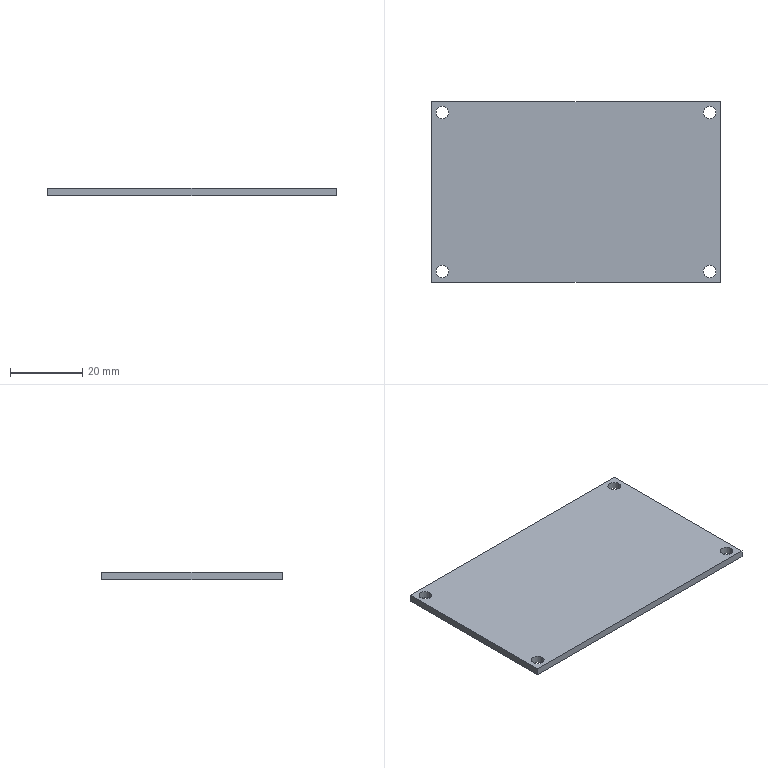Part | SolidWorks | features ICE 19, MoveFace 6, Fillet 2, BaseBody 1 | 1 solid | 14 faces | box 80 x 50 x 2 mm | volume 7923 mm3 | cylinder 8 | plane 6 | commonest cylinder face diameters 3.5 x8
STEP:
#1=CARTESIAN_POINT('',(-42.75,130.634,-3.2));
#2=VERTEX_POINT('',#1);
#3=CARTESIAN_POINT('',(-46.25,130.634,-3.2));
#4=VERTEX_POINT('',#3);
#5=CARTESIAN_POINT('',(-44.5,130.634,-3.2));
#6=DIRECTION('',(0.,0.,-1.));
#7=DIRECTION('',(-1.,0.,0.));
#8=AXIS2_PLACEMENT_3D('',#5,#6,#7);
#9=CIRCLE('',#8,1.75);
#10=EDGE_CURVE('',#2,#4,#9,.T.);
#11=ORIENTED_EDGE('',*,*,#10,.T.);
#12=CARTESIAN_POINT('',(-46.25,130.634,-1.2));
#13=VERTEX_POINT('',#12);
#14=CARTESIAN_POINT('',(-46.25,130.634,-3.2));
#15=DIRECTION('',(0.,0.,1.));
#16=VECTOR('',#15,1000.);
#17=LINE('',#14,#16);
#18=EDGE_CURVE('',#4,#13,#17,.T.);
#19=ORIENTED_EDGE('',*,*,#18,.T.);
#20=CARTESIAN_POINT('',(-42.75,130.634,-1.2));
#21=VERTEX_POINT('',#20);
#22=CARTESIAN_POINT('',(-44.5,130.634,-1.2));
#23=DIRECTION('',(0.,0.,-1.));
#24=DIRECTION('',(-1.,0.,0.));
#25=AXIS2_PLACEMENT_3D('',#22,#23,#24);
#26=CIRCLE('',#25,1.75);
#27=EDGE_CURVE('',#21,#13,#26,.T.);
#28=ORIENTED_EDGE('',*,*,#27,.F.);
#29=CARTESIAN_POINT('',(-42.75,130.634,-3.2));
#30=DIRECTION('',(0.,0.,1.));
#31=VECTOR('',#30,1000.);
#32=LINE('',#29,#31);
#33=EDGE_CURVE('',#2,#21,#32,.T.);
#34=ORIENTED_EDGE('',*,*,#33,.F.);
#35=EDGE_LOOP('',(#11,#19,#28,#34));
#36=FACE_OUTER_BOUND('',#35,.T.);
#37=CARTESIAN_POINT('',(-44.5,130.634,-3.2));
#38=DIRECTION('',(0.,0.,1.));
#39=DIRECTION('',(1.,0.,0.));
#40=AXIS2_PLACEMENT_3D('',#37,#38,#39);
#41=CYLINDRICAL_SURFACE('',#40,1.75);
#42=ADVANCED_FACE('',(#36),#41,.F.);
#43=CARTESIAN_POINT('',(-42.75,174.634,-3.2));
#44=VERTEX_POINT('',#43);
#45=CARTESIAN_POINT('',(-46.25,174.634,-3.2));
#46=VERTEX_POINT('',#45);
#47=CARTESIAN_POINT('',(-44.5,174.634,-3.2));
#48=DIRECTION('',(0.,0.,-1.));
#49=DIRECTION('',(-1.,0.,0.));
#50=AXIS2_PLACEMENT_3D('',#47,#48,#49);
#51=CIRCLE('',#50,1.75);
#52=EDGE_CURVE('',#44,#46,#51,.T.);
#53=ORIENTED_EDGE('',*,*,#52,.T.);
#54=CARTESIAN_POINT('',(-46.25,174.634,-1.2));
#55=VERTEX_POINT('',#54);
#56=CARTESIAN_POINT('',(-46.25,174.634,-3.2));
#57=DIRECTION('',(0.,0.,1.));
#58=VECTOR('',#57,1000.);
#59=LINE('',#56,#58);
#60=EDGE_CURVE('',#46,#55,#59,.T.);
#61=ORIENTED_EDGE('',*,*,#60,.T.);
#62=CARTESIAN_POINT('',(-42.75,174.634,-1.2));
#63=VERTEX_POINT('',#62);
#64=CARTESIAN_POINT('',(-44.5,174.634,-1.2));
#65=DIRECTION('',(0.,0.,-1.));
#66=DIRECTION('',(-1.,0.,0.));
#67=AXIS2_PLACEMENT_3D('',#64,#65,#66);
#68=CIRCLE('',#67,1.75);
#69=EDGE_CURVE('',#63,#55,#68,.T.);
#70=ORIENTED_EDGE('',*,*,#69,.F.);
#71=CARTESIAN_POINT('',(-42.75,174.634,-3.2));
#72=DIRECTION('',(0.,0.,1.));
#73=VECTOR('',#72,1000.);
#74=LINE('',#71,#73);
#75=EDGE_CURVE('',#44,#63,#74,.T.);
#76=ORIENTED_EDGE('',*,*,#75,.F.);
#77=EDGE_LOOP('',(#53,#61,#70,#76));
#78=FACE_OUTER_BOUND('',#77,.T.);
#79=CARTESIAN_POINT('',(-44.5,174.634,-3.2));
#80=DIRECTION('',(0.,0.,1.));
#81=DIRECTION('',(1.,0.,0.));
#82=AXIS2_PLACEMENT_3D('',#79,#80,#81);
#83=CYLINDRICAL_SURFACE('',#82,1.75);
#84=ADVANCED_FACE('',(#78),#83,.F.);
#85=CARTESIAN_POINT('',(31.25,174.634,-3.2));
#86=VERTEX_POINT('',#85);
#87=CARTESIAN_POINT('',(27.75,174.634,-3.2));
#88=VERTEX_POINT('',#87);
#89=CARTESIAN_POINT('',(29.5,174.634,-3.2));
#90=DIRECTION('',(0.,0.,-1.));
#91=DIRECTION('',(-1.,0.,0.));
#92=AXIS2_PLACEMENT_3D('',#89,#90,#91);
#93=CIRCLE('',#92,1.75);
#94=EDGE_CURVE('',#86,#88,#93,.T.);
#95=ORIENTED_EDGE('',*,*,#94,.T.);
#96=CARTESIAN_POINT('',(27.75,174.634,-1.2));
#97=VERTEX_POINT('',#96);
#98=CARTESIAN_POINT('',(27.75,174.634,-3.2));
#99=DIRECTION('',(0.,0.,1.));
#100=VECTOR('',#99,1000.);
#101=LINE('',#98,#100);
#102=EDGE_CURVE('',#88,#97,#101,.T.);
#103=ORIENTED_EDGE('',*,*,#102,.T.);
#104=CARTESIAN_POINT('',(31.25,174.634,-1.2));
#105=VERTEX_POINT('',#104);
#106=CARTESIAN_POINT('',(29.5,174.634,-1.2));
#107=DIRECTION('',(0.,0.,-1.));
#108=DIRECTION('',(-1.,0.,0.));
#109=AXIS2_PLACEMENT_3D('',#106,#107,#108);
#110=CIRCLE('',#109,1.75);
#111=EDGE_CURVE('',#105,#97,#110,.T.);
#112=ORIENTED_EDGE('',*,*,#111,.F.);
#113=CARTESIAN_POINT('',(31.25,174.634,-3.2));
#114=DIRECTION('',(0.,0.,1.));
#115=VECTOR('',#114,1000.);
#116=LINE('',#113,#115);
#117=EDGE_CURVE('',#86,#105,#116,.T.);
#118=ORIENTED_EDGE('',*,*,#117,.F.);
#119=EDGE_LOOP('',(#95,#103,#112,#118));
#120=FACE_OUTER_BOUND('',#119,.T.);
#121=CARTESIAN_POINT('',(29.5,174.634,-3.2));
#122=DIRECTION('',(0.,0.,1.));
#123=DIRECTION('',(1.,0.,0.));
#124=AXIS2_PLACEMENT_3D('',#121,#122,#123);
#125=CYLINDRICAL_SURFACE('',#124,1.75);
#126=ADVANCED_FACE('',(#120),#125,.F.);
#127=CARTESIAN_POINT('',(31.25,130.634,-3.2));
#128=VERTEX_POINT('',#127);
#129=CARTESIAN_POINT('',(27.75,130.634,-3.2));
#130=VERTEX_POINT('',#129);
#131=CARTESIAN_POINT('',(29.5,130.634,-3.2));
#132=DIRECTION('',(0.,0.,-1.));
#133=DIRECTION('',(-1.,0.,0.));
#134=AXIS2_PLACEMENT_3D('',#131,#132,#133);
#135=CIRCLE('',#134,1.75);
#136=EDGE_CURVE('',#128,#130,#135,.T.);
#137=ORIENTED_EDGE('',*,*,#136,.T.);
#138=CARTESIAN_POINT('',(27.75,130.634,-1.2));
#139=VERTEX_POINT('',#138);
#140=CARTESIAN_POINT('',(27.75,130.634,-3.2));
#141=DIRECTION('',(0.,0.,1.));
#142=VECTOR('',#141,1000.);
#143=LINE('',#140,#142);
#144=EDGE_CURVE('',#130,#139,#143,.T.);
#145=ORIENTED_EDGE('',*,*,#144,.T.);
#146=CARTESIAN_POINT('',(31.25,130.634,-1.2));
#147=VERTEX_POINT('',#146);
#148=CARTESIAN_POINT('',(29.5,130.634,-1.2));
#149=DIRECTION('',(0.,0.,-1.));
#150=DIRECTION('',(-1.,0.,0.));
#151=AXIS2_PLACEMENT_3D('',#148,#149,#150);
#152=CIRCLE('',#151,1.75);
#153=EDGE_CURVE('',#147,#139,#152,.T.);
#154=ORIENTED_EDGE('',*,*,#153,.F.);
#155=CARTESIAN_POINT('',(31.25,130.634,-3.2));
#156=DIRECTION('',(0.,0.,1.));
#157=VECTOR('',#156,1000.);
#158=LINE('',#155,#157);
#159=EDGE_CURVE('',#128,#147,#158,.T.);
#160=ORIENTED_EDGE('',*,*,#159,.F.);
#161=EDGE_LOOP('',(#137,#145,#154,#160));
#162=FACE_OUTER_BOUND('',#161,.T.);
#163=CARTESIAN_POINT('',(29.5,130.634,-3.2));
#164=DIRECTION('',(0.,0.,1.));
#165=DIRECTION('',(1.,0.,0.));
#166=AXIS2_PLACEMENT_3D('',#163,#164,#165);
#167=CYLINDRICAL_SURFACE('',#166,1.75);
#168=ADVANCED_FACE('',(#162),#167,.F.);
#169=ORIENTED_EDGE('',*,*,#52,.F.);
#170=CARTESIAN_POINT('',(-44.5,174.634,-3.2));
#171=DIRECTION('',(0.,0.,-1.));
#172=DIRECTION('',(-1.,0.,0.));
#173=AXIS2_PLACEMENT_3D('',#170,#171,#172);
#174=CIRCLE('',#173,1.75);
#175=EDGE_CURVE('',#46,#44,#174,.T.);
#176=ORIENTED_EDGE('',*,*,#175,.F.);
#177=EDGE_LOOP('',(#169,#176));
#178=FACE_BOUND('',#177,.T.);
#179=ORIENTED_EDGE('',*,*,#136,.F.);
#180=CARTESIAN_POINT('',(29.5,130.634,-3.2));
#181=DIRECTION('',(0.,0.,-1.));
#182=DIRECTION('',(-1.,0.,0.));
#183=AXIS2_PLACEMENT_3D('',#180,#181,#182);
#184=CIRCLE('',#183,1.75);
#185=EDGE_CURVE('',#130,#128,#184,.T.);
#186=ORIENTED_EDGE('',*,*,#185,.F.);
#187=EDGE_LOOP('',(#179,#186));
#188=FACE_BOUND('',#187,.T.);
#189=CARTESIAN_POINT('',(-47.5,127.634,-3.2));
#190=VERTEX_POINT('',#189);
#191=CARTESIAN_POINT('',(-47.5,177.634,-3.2));
#192=VERTEX_POINT('',#191);
#193=CARTESIAN_POINT('',(-47.5,127.634,-3.2));
#194=DIRECTION('',(0.,1.,0.));
#195=VECTOR('',#194,1000.);
#196=LINE('',#193,#195);
#197=EDGE_CURVE('',#190,#192,#196,.T.);
#198=ORIENTED_EDGE('',*,*,#197,.T.);
#199=CARTESIAN_POINT('',(32.5,177.634,-3.2));
#200=VERTEX_POINT('',#199);
#201=CARTESIAN_POINT('',(-47.5,177.634,-3.2));
#202=DIRECTION('',(1.,0.,0.));
#203=VECTOR('',#202,1000.);
#204=LINE('',#201,#203);
#205=EDGE_CURVE('',#192,#200,#204,.T.);
#206=ORIENTED_EDGE('',*,*,#205,.T.);
#207=CARTESIAN_POINT('',(32.5,127.634,-3.2));
#208=VERTEX_POINT('',#207);
#209=CARTESIAN_POINT('',(32.5,127.634,-3.2));
#210=DIRECTION('',(0.,-1.,0.));
#211=VECTOR('',#210,1000.);
#212=LINE('',#209,#211);
#213=EDGE_CURVE('',#200,#208,#212,.T.);
#214=ORIENTED_EDGE('',*,*,#213,.T.);
#215=CARTESIAN_POINT('',(-47.5,127.634,-3.2));
#216=DIRECTION('',(-1.,0.,0.));
#217=VECTOR('',#216,1000.);
#218=LINE('',#215,#217);
#219=EDGE_CURVE('',#208,#190,#218,.T.);
#220=ORIENTED_EDGE('',*,*,#219,.T.);
#221=EDGE_LOOP('',(#198,#206,#214,#220));
#222=FACE_OUTER_BOUND('',#221,.T.);
#223=ORIENTED_EDGE('',*,*,#94,.F.);
#224=CARTESIAN_POINT('',(29.5,174.634,-3.2));
#225=DIRECTION('',(0.,0.,-1.));
#226=DIRECTION('',(-1.,0.,0.));
#227=AXIS2_PLACEMENT_3D('',#224,#225,#226);
#228=CIRCLE('',#227,1.75);
#229=EDGE_CURVE('',#88,#86,#228,.T.);
#230=ORIENTED_EDGE('',*,*,#229,.F.);
#231=EDGE_LOOP('',(#223,#230));
#232=FACE_BOUND('',#231,.T.);
#233=ORIENTED_EDGE('',*,*,#10,.F.);
#234=CARTESIAN_POINT('',(-44.5,130.634,-3.2));
#235=DIRECTION('',(0.,0.,-1.));
#236=DIRECTION('',(-1.,0.,0.));
#237=AXIS2_PLACEMENT_3D('',#234,#235,#236);
#238=CIRCLE('',#237,1.75);
#239=EDGE_CURVE('',#4,#2,#238,.T.);
#240=ORIENTED_EDGE('',*,*,#239,.F.);
#241=EDGE_LOOP('',(#233,#240));
#242=FACE_BOUND('',#241,.T.);
#243=CARTESIAN_POINT('',(0.,0.,-3.2));
#244=DIRECTION('',(0.,0.,-1.));
#245=DIRECTION('',(-1.,0.,0.));
#246=AXIS2_PLACEMENT_3D('',#243,#244,#245);
#247=PLANE('',#246);
#248=ADVANCED_FACE('',(#178,#188,#222,#232,#242),#247,.T.);
#249=CARTESIAN_POINT('',(-47.5,127.634,-1.2));
#250=VERTEX_POINT('',#249);
#251=CARTESIAN_POINT('',(-47.5,177.634,-1.2));
#252=VERTEX_POINT('',#251);
#253=CARTESIAN_POINT('',(-47.5,127.634,-1.2));
#254=DIRECTION('',(0.,1.,0.));
#255=VECTOR('',#254,1000.);
#256=LINE('',#253,#255);
#257=EDGE_CURVE('',#250,#252,#256,.T.);
#258=ORIENTED_EDGE('',*,*,#257,.F.);
#259=CARTESIAN_POINT('',(32.5,127.634,-1.2));
#260=VERTEX_POINT('',#259);
#261=CARTESIAN_POINT('',(-47.5,127.634,-1.2));
#262=DIRECTION('',(-1.,0.,0.));
#263=VECTOR('',#262,1000.);
#264=LINE('',#261,#263);
#265=EDGE_CURVE('',#260,#250,#264,.T.);
#266=ORIENTED_EDGE('',*,*,#265,.F.);
#267=CARTESIAN_POINT('',(32.5,177.634,-1.2));
#268=VERTEX_POINT('',#267);
#269=CARTESIAN_POINT('',(32.5,127.634,-1.2));
#270=DIRECTION('',(0.,-1.,0.));
#271=VECTOR('',#270,1000.);
#272=LINE('',#269,#271);
#273=EDGE_CURVE('',#268,#260,#272,.T.);
#274=ORIENTED_EDGE('',*,*,#273,.F.);
#275=CARTESIAN_POINT('',(-47.5,177.634,-1.2));
#276=DIRECTION('',(1.,0.,0.));
#277=VECTOR('',#276,1000.);
#278=LINE('',#275,#277);
#279=EDGE_CURVE('',#252,#268,#278,.T.);
#280=ORIENTED_EDGE('',*,*,#279,.F.);
#281=EDGE_LOOP('',(#258,#266,#274,#280));
#282=FACE_OUTER_BOUND('',#281,.T.);
#283=ORIENTED_EDGE('',*,*,#153,.T.);
#284=CARTESIAN_POINT('',(29.5,130.634,-1.2));
#285=DIRECTION('',(0.,0.,-1.));
#286=DIRECTION('',(-1.,0.,0.));
#287=AXIS2_PLACEMENT_3D('',#284,#285,#286);
#288=CIRCLE('',#287,1.75);
#289=EDGE_CURVE('',#139,#147,#288,.T.);
#290=ORIENTED_EDGE('',*,*,#289,.T.);
#291=EDGE_LOOP('',(#283,#290));
#292=FACE_BOUND('',#291,.T.);
#293=ORIENTED_EDGE('',*,*,#111,.T.);
#294=CARTESIAN_POINT('',(29.5,174.634,-1.2));
#295=DIRECTION('',(0.,0.,-1.));
#296=DIRECTION('',(-1.,0.,0.));
#297=AXIS2_PLACEMENT_3D('',#294,#295,#296);
#298=CIRCLE('',#297,1.75);
#299=EDGE_CURVE('',#97,#105,#298,.T.);
#300=ORIENTED_EDGE('',*,*,#299,.T.);
#301=EDGE_LOOP('',(#293,#300));
#302=FACE_BOUND('',#301,.T.);
#303=ORIENTED_EDGE('',*,*,#69,.T.);
#304=CARTESIAN_POINT('',(-44.5,174.634,-1.2));
#305=DIRECTION('',(0.,0.,-1.));
#306=DIRECTION('',(-1.,0.,0.));
#307=AXIS2_PLACEMENT_3D('',#304,#305,#306);
#308=CIRCLE('',#307,1.75);
#309=EDGE_CURVE('',#55,#63,#308,.T.);
#310=ORIENTED_EDGE('',*,*,#309,.T.);
#311=EDGE_LOOP('',(#303,#310));
#312=FACE_BOUND('',#311,.T.);
#313=ORIENTED_EDGE('',*,*,#27,.T.);
#314=CARTESIAN_POINT('',(-44.5,130.634,-1.2));
#315=DIRECTION('',(0.,0.,-1.));
#316=DIRECTION('',(-1.,0.,0.));
#317=AXIS2_PLACEMENT_3D('',#314,#315,#316);
#318=CIRCLE('',#317,1.75);
#319=EDGE_CURVE('',#13,#21,#318,.T.);
#320=ORIENTED_EDGE('',*,*,#319,.T.);
#321=EDGE_LOOP('',(#313,#320));
#322=FACE_BOUND('',#321,.T.);
#323=CARTESIAN_POINT('',(0.,0.,-1.2));
#324=DIRECTION('',(0.,0.,-1.));
#325=DIRECTION('',(-1.,0.,0.));
#326=AXIS2_PLACEMENT_3D('',#323,#324,#325);
#327=PLANE('',#326);
#328=ADVANCED_FACE('',(#282,#292,#302,#312,#322),#327,.F.);
#329=ORIENTED_EDGE('',*,*,#257,.T.);
#330=CARTESIAN_POINT('',(-47.5,177.634,-3.2));
#331=DIRECTION('',(0.,0.,1.));
#332=VECTOR('',#331,1000.);
#333=LINE('',#330,#332);
#334=EDGE_CURVE('',#192,#252,#333,.T.);
#335=ORIENTED_EDGE('',*,*,#334,.F.);
#336=ORIENTED_EDGE('',*,*,#197,.F.);
#337=CARTESIAN_POINT('',(-47.5,127.634,-3.2));
#338=DIRECTION('',(0.,0.,1.));
#339=VECTOR('',#338,1000.);
#340=LINE('',#337,#339);
#341=EDGE_CURVE('',#190,#250,#340,.T.);
#342=ORIENTED_EDGE('',*,*,#341,.T.);
#343=EDGE_LOOP('',(#329,#335,#336,#342));
#344=FACE_OUTER_BOUND('',#343,.T.);
#345=CARTESIAN_POINT('',(-47.5,127.634,-3.2));
#346=DIRECTION('',(1.,0.,0.));
#347=DIRECTION('',(0.,1.,0.));
#348=AXIS2_PLACEMENT_3D('',#345,#346,#347);
#349=PLANE('',#348);
#350=ADVANCED_FACE('',(#344),#349,.F.);
#351=ORIENTED_EDGE('',*,*,#279,.T.);
#352=CARTESIAN_POINT('',(32.5,177.634,-3.2));
#353=DIRECTION('',(0.,0.,1.));
#354=VECTOR('',#353,1000.);
#355=LINE('',#352,#354);
#356=EDGE_CURVE('',#200,#268,#355,.T.);
#357=ORIENTED_EDGE('',*,*,#356,.F.);
#358=ORIENTED_EDGE('',*,*,#205,.F.);
#359=ORIENTED_EDGE('',*,*,#334,.T.);
#360=EDGE_LOOP('',(#351,#357,#358,#359));
#361=FACE_OUTER_BOUND('',#360,.T.);
#362=CARTESIAN_POINT('',(-47.5,177.634,-3.2));
#363=DIRECTION('',(0.,-1.,0.));
#364=DIRECTION('',(0.,0.,-1.));
#365=AXIS2_PLACEMENT_3D('',#362,#363,#364);
#366=PLANE('',#365);
#367=ADVANCED_FACE('',(#361),#366,.F.);
#368=ORIENTED_EDGE('',*,*,#273,.T.);
#369=CARTESIAN_POINT('',(32.5,127.634,-3.2));
#370=DIRECTION('',(0.,0.,1.));
#371=VECTOR('',#370,1000.);
#372=LINE('',#369,#371);
#373=EDGE_CURVE('',#208,#260,#372,.T.);
#374=ORIENTED_EDGE('',*,*,#373,.F.);
#375=ORIENTED_EDGE('',*,*,#213,.F.);
#376=ORIENTED_EDGE('',*,*,#356,.T.);
#377=EDGE_LOOP('',(#368,#374,#375,#376));
#378=FACE_OUTER_BOUND('',#377,.T.);
#379=CARTESIAN_POINT('',(32.5,127.634,-3.2));
#380=DIRECTION('',(-1.,0.,0.));
#381=DIRECTION('',(0.,-1.,0.));
#382=AXIS2_PLACEMENT_3D('',#379,#380,#381);
#383=PLANE('',#382);
#384=ADVANCED_FACE('',(#378),#383,.F.);
#385=ORIENTED_EDGE('',*,*,#265,.T.);
#386=ORIENTED_EDGE('',*,*,#341,.F.);
#387=ORIENTED_EDGE('',*,*,#219,.F.);
#388=ORIENTED_EDGE('',*,*,#373,.T.);
#389=EDGE_LOOP('',(#385,#386,#387,#388));
#390=FACE_OUTER_BOUND('',#389,.T.);
#391=CARTESIAN_POINT('',(-47.5,127.634,-3.2));
#392=DIRECTION('',(0.,1.,0.));
#393=DIRECTION('',(0.,0.,1.));
#394=AXIS2_PLACEMENT_3D('',#391,#392,#393);
#395=PLANE('',#394);
#396=ADVANCED_FACE('',(#390),#395,.F.);
#397=ORIENTED_EDGE('',*,*,#144,.F.);
#398=ORIENTED_EDGE('',*,*,#185,.T.);
#399=ORIENTED_EDGE('',*,*,#159,.T.);
#400=ORIENTED_EDGE('',*,*,#289,.F.);
#401=EDGE_LOOP('',(#397,#398,#399,#400));
#402=FACE_OUTER_BOUND('',#401,.T.);
#403=CARTESIAN_POINT('',(29.5,130.634,-3.2));
#404=DIRECTION('',(0.,0.,1.));
#405=DIRECTION('',(1.,0.,0.));
#406=AXIS2_PLACEMENT_3D('',#403,#404,#405);
#407=CYLINDRICAL_SURFACE('',#406,1.75);
#408=ADVANCED_FACE('',(#402),#407,.F.);
#409=ORIENTED_EDGE('',*,*,#102,.F.);
#410=ORIENTED_EDGE('',*,*,#229,.T.);
#411=ORIENTED_EDGE('',*,*,#117,.T.);
#412=ORIENTED_EDGE('',*,*,#299,.F.);
#413=EDGE_LOOP('',(#409,#410,#411,#412));
#414=FACE_OUTER_BOUND('',#413,.T.);
#415=CARTESIAN_POINT('',(29.5,174.634,-3.2));
#416=DIRECTION('',(0.,0.,1.));
#417=DIRECTION('',(1.,0.,0.));
#418=AXIS2_PLACEMENT_3D('',#415,#416,#417);
#419=CYLINDRICAL_SURFACE('',#418,1.75);
#420=ADVANCED_FACE('',(#414),#419,.F.);
#421=ORIENTED_EDGE('',*,*,#60,.F.);
#422=ORIENTED_EDGE('',*,*,#175,.T.);
#423=ORIENTED_EDGE('',*,*,#75,.T.);
#424=ORIENTED_EDGE('',*,*,#309,.F.);
#425=EDGE_LOOP('',(#421,#422,#423,#424));
#426=FACE_OUTER_BOUND('',#425,.T.);
#427=CARTESIAN_POINT('',(-44.5,174.634,-3.2));
#428=DIRECTION('',(0.,0.,1.));
#429=DIRECTION('',(1.,0.,0.));
#430=AXIS2_PLACEMENT_3D('',#427,#428,#429);
#431=CYLINDRICAL_SURFACE('',#430,1.75);
#432=ADVANCED_FACE('',(#426),#431,.F.);
#433=ORIENTED_EDGE('',*,*,#18,.F.);
#434=ORIENTED_EDGE('',*,*,#239,.T.);
#435=ORIENTED_EDGE('',*,*,#33,.T.);
#436=ORIENTED_EDGE('',*,*,#319,.F.);
#437=EDGE_LOOP('',(#433,#434,#435,#436));
#438=FACE_OUTER_BOUND('',#437,.T.);
#439=CARTESIAN_POINT('',(-44.5,130.634,-3.2));
#440=DIRECTION('',(0.,0.,1.));
#441=DIRECTION('',(1.,0.,0.));
#442=AXIS2_PLACEMENT_3D('',#439,#440,#441);
#443=CYLINDRICAL_SURFACE('',#442,1.75);
#444=ADVANCED_FACE('',(#438),#443,.F.);
#445=CLOSED_SHELL('',(#42,#84,#126,#168,#248,#328,#350,#367,#384,#396,#408,#420,#432,#444));
#446=MANIFOLD_SOLID_BREP('',#445);
#447=CARTESIAN_POINT('',(0.,0.,0.));
#448=DIRECTION('',(0.,0.,1.));
#449=DIRECTION('',(1.,0.,0.));
#450=AXIS2_PLACEMENT_3D('',#447,#448,#449);
#451=(LENGTH_UNIT()NAMED_UNIT(*)SI_UNIT(.MILLI.,.METRE.));
#452=UNCERTAINTY_MEASURE_WITH_UNIT(LENGTH_MEASURE(0.00001),#451,'','');
#453=(NAMED_UNIT(*)PLANE_ANGLE_UNIT()SI_UNIT($,.RADIAN.));
#454=(NAMED_UNIT(*)SI_UNIT($,.STERADIAN.)SOLID_ANGLE_UNIT());
#455=(GEOMETRIC_REPRESENTATION_CONTEXT(3)GLOBAL_UNCERTAINTY_ASSIGNED_CONTEXT((#452))GLOBAL_UNIT_ASSIGNED_CONTEXT((#451,#453,#454))REPRESENTATION_CONTEXT('',''));
#456=ADVANCED_BREP_SHAPE_REPRESENTATION('',(#446,#450),#455);